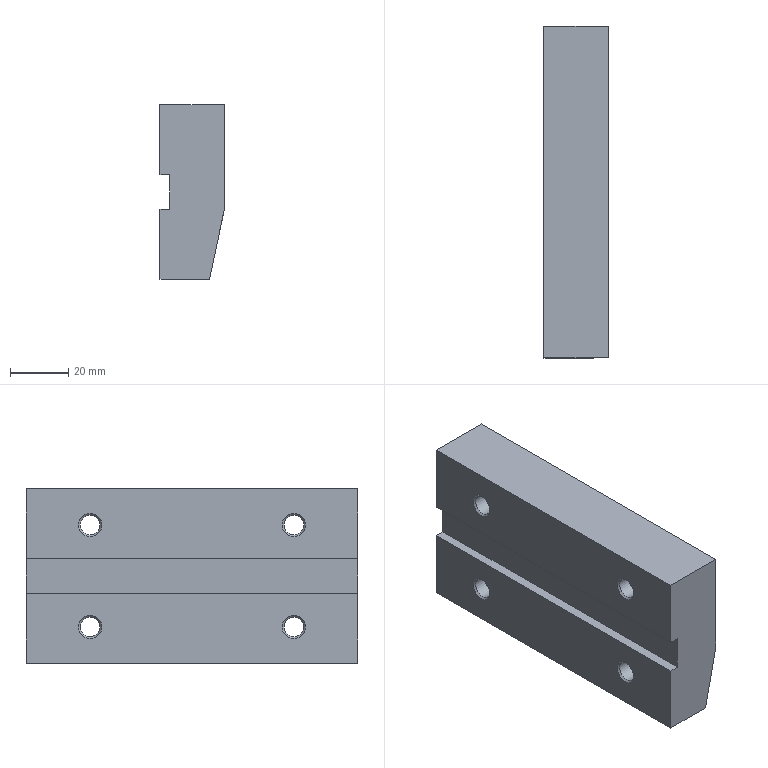Part | NX | features SIMPLE HOLE 4, SYMBOLIC_THREAD 4, DATUM_CSYS 3, SKETCH 2, EXTRUDE 1, HOLE PACKAGE 1 | 1 solid | 23 faces | box 22 x 114 x 60 mm | volume 136204 mm3 | plane 11 | cone 6 | cylinder 4 | spline 2 | commonest cylinder face diameters 6.8 x4
STEP:
#1=CARTESIAN_POINT('',(0.,92.,-51.5));
#2=VERTEX_POINT('',#1);
#3=CARTESIAN_POINT('',(0.,92.,-47.5));
#4=DIRECTION('',(1.,0.,0.));
#5=DIRECTION('',(0.,0.,-1.));
#6=AXIS2_PLACEMENT_3D('',#3,#4,#5);
#7=CIRCLE('',#6,4.);
#8=EDGE_CURVE('',#2,#2,#7,.T.);
#9=ORIENTED_EDGE('',*,*,#8,.T.);
#10=EDGE_LOOP('',(#9));
#11=FACE_BOUND('',#10,.T.);
#12=CARTESIAN_POINT('',(0.,22.,-51.5));
#13=VERTEX_POINT('',#12);
#14=CARTESIAN_POINT('',(0.,22.,-47.5));
#15=DIRECTION('',(1.,0.,0.));
#16=DIRECTION('',(0.,0.,-1.));
#17=AXIS2_PLACEMENT_3D('',#14,#15,#16);
#18=CIRCLE('',#17,4.);
#19=EDGE_CURVE('',#13,#13,#18,.T.);
#20=ORIENTED_EDGE('',*,*,#19,.T.);
#21=EDGE_LOOP('',(#20));
#22=FACE_BOUND('',#21,.T.);
#23=CARTESIAN_POINT('',(0.,0.,-60.));
#24=VERTEX_POINT('',#23);
#25=CARTESIAN_POINT('',(0.,0.,-36.));
#26=VERTEX_POINT('',#25);
#27=CARTESIAN_POINT('',(0.,0.,-60.));
#28=DIRECTION('',(0.,0.,1.));
#29=VECTOR('',#28,1000.);
#30=LINE('',#27,#29);
#31=EDGE_CURVE('',#24,#26,#30,.T.);
#32=ORIENTED_EDGE('',*,*,#31,.T.);
#33=CARTESIAN_POINT('',(0.,114.,-36.));
#34=VERTEX_POINT('',#33);
#35=CARTESIAN_POINT('',(0.,114.,-36.));
#36=DIRECTION('',(0.,-1.,0.));
#37=VECTOR('',#36,1000.);
#38=LINE('',#35,#37);
#39=EDGE_CURVE('',#34,#26,#38,.T.);
#40=ORIENTED_EDGE('',*,*,#39,.F.);
#41=CARTESIAN_POINT('',(0.,114.,-60.));
#42=VERTEX_POINT('',#41);
#43=CARTESIAN_POINT('',(0.,114.,-60.));
#44=DIRECTION('',(0.,0.,1.));
#45=VECTOR('',#44,1000.);
#46=LINE('',#43,#45);
#47=EDGE_CURVE('',#42,#34,#46,.T.);
#48=ORIENTED_EDGE('',*,*,#47,.F.);
#49=CARTESIAN_POINT('',(0.,114.,-60.));
#50=DIRECTION('',(0.,-1.,0.));
#51=VECTOR('',#50,1000.);
#52=LINE('',#49,#51);
#53=EDGE_CURVE('',#42,#24,#52,.T.);
#54=ORIENTED_EDGE('',*,*,#53,.T.);
#55=EDGE_LOOP('',(#32,#40,#48,#54));
#56=FACE_BOUND('',#55,.T.);
#57=CARTESIAN_POINT('',(0.,114.,-60.));
#58=DIRECTION('',(1.,0.,0.));
#59=DIRECTION('',(0.,0.,-1.));
#60=AXIS2_PLACEMENT_3D('',#57,#58,#59);
#61=PLANE('',#60);
#62=ADVANCED_FACE('',(#11,#22,#56),#61,.F.);
#63=CARTESIAN_POINT('',(3.3,0.,-36.));
#64=VERTEX_POINT('',#63);
#65=CARTESIAN_POINT('',(0.,0.,-36.));
#66=DIRECTION('',(1.,0.,0.));
#67=VECTOR('',#66,1000.);
#68=LINE('',#65,#67);
#69=EDGE_CURVE('',#26,#64,#68,.T.);
#70=ORIENTED_EDGE('',*,*,#69,.T.);
#71=CARTESIAN_POINT('',(3.3,114.,-36.));
#72=VERTEX_POINT('',#71);
#73=CARTESIAN_POINT('',(3.3,114.,-36.));
#74=DIRECTION('',(0.,-1.,0.));
#75=VECTOR('',#74,1000.);
#76=LINE('',#73,#75);
#77=EDGE_CURVE('',#72,#64,#76,.T.);
#78=ORIENTED_EDGE('',*,*,#77,.F.);
#79=CARTESIAN_POINT('',(0.,114.,-36.));
#80=DIRECTION('',(1.,0.,0.));
#81=VECTOR('',#80,1000.);
#82=LINE('',#79,#81);
#83=EDGE_CURVE('',#34,#72,#82,.T.);
#84=ORIENTED_EDGE('',*,*,#83,.F.);
#85=ORIENTED_EDGE('',*,*,#39,.T.);
#86=EDGE_LOOP('',(#70,#78,#84,#85));
#87=FACE_BOUND('',#86,.T.);
#88=CARTESIAN_POINT('',(0.,114.,-36.));
#89=DIRECTION('',(0.,0.,-1.));
#90=DIRECTION('',(-1.,0.,0.));
#91=AXIS2_PLACEMENT_3D('',#88,#89,#90);
#92=PLANE('',#91);
#93=ADVANCED_FACE('',(#87),#92,.F.);
#94=CARTESIAN_POINT('',(3.3,0.,-24.));
#95=VERTEX_POINT('',#94);
#96=CARTESIAN_POINT('',(3.3,0.,-36.));
#97=DIRECTION('',(0.,0.,1.));
#98=VECTOR('',#97,1000.);
#99=LINE('',#96,#98);
#100=EDGE_CURVE('',#64,#95,#99,.T.);
#101=ORIENTED_EDGE('',*,*,#100,.T.);
#102=CARTESIAN_POINT('',(3.3,114.,-24.));
#103=VERTEX_POINT('',#102);
#104=CARTESIAN_POINT('',(3.3,114.,-24.));
#105=DIRECTION('',(0.,-1.,0.));
#106=VECTOR('',#105,1000.);
#107=LINE('',#104,#106);
#108=EDGE_CURVE('',#103,#95,#107,.T.);
#109=ORIENTED_EDGE('',*,*,#108,.F.);
#110=CARTESIAN_POINT('',(3.3,114.,-36.));
#111=DIRECTION('',(0.,0.,1.));
#112=VECTOR('',#111,1000.);
#113=LINE('',#110,#112);
#114=EDGE_CURVE('',#72,#103,#113,.T.);
#115=ORIENTED_EDGE('',*,*,#114,.F.);
#116=ORIENTED_EDGE('',*,*,#77,.T.);
#117=EDGE_LOOP('',(#101,#109,#115,#116));
#118=FACE_BOUND('',#117,.T.);
#119=CARTESIAN_POINT('',(3.3,114.,-36.));
#120=DIRECTION('',(1.,0.,0.));
#121=DIRECTION('',(0.,0.,-1.));
#122=AXIS2_PLACEMENT_3D('',#119,#120,#121);
#123=PLANE('',#122);
#124=ADVANCED_FACE('',(#118),#123,.F.);
#125=CARTESIAN_POINT('',(0.,0.,-24.));
#126=VERTEX_POINT('',#125);
#127=CARTESIAN_POINT('',(3.3,0.,-24.));
#128=DIRECTION('',(-1.,0.,0.));
#129=VECTOR('',#128,1000.);
#130=LINE('',#127,#129);
#131=EDGE_CURVE('',#95,#126,#130,.T.);
#132=ORIENTED_EDGE('',*,*,#131,.T.);
#133=CARTESIAN_POINT('',(0.,114.,-24.));
#134=VERTEX_POINT('',#133);
#135=CARTESIAN_POINT('',(0.,114.,-24.));
#136=DIRECTION('',(0.,-1.,0.));
#137=VECTOR('',#136,1000.);
#138=LINE('',#135,#137);
#139=EDGE_CURVE('',#134,#126,#138,.T.);
#140=ORIENTED_EDGE('',*,*,#139,.F.);
#141=CARTESIAN_POINT('',(3.3,114.,-24.));
#142=DIRECTION('',(-1.,0.,0.));
#143=VECTOR('',#142,1000.);
#144=LINE('',#141,#143);
#145=EDGE_CURVE('',#103,#134,#144,.T.);
#146=ORIENTED_EDGE('',*,*,#145,.F.);
#147=ORIENTED_EDGE('',*,*,#108,.T.);
#148=EDGE_LOOP('',(#132,#140,#146,#147));
#149=FACE_BOUND('',#148,.T.);
#150=CARTESIAN_POINT('',(3.3,114.,-24.));
#151=DIRECTION('',(0.,0.,1.));
#152=DIRECTION('',(1.,0.,0.));
#153=AXIS2_PLACEMENT_3D('',#150,#151,#152);
#154=PLANE('',#153);
#155=ADVANCED_FACE('',(#149),#154,.F.);
#156=CARTESIAN_POINT('',(0.,92.,-16.5));
#157=VERTEX_POINT('',#156);
#158=CARTESIAN_POINT('',(0.,92.,-12.5));
#159=DIRECTION('',(1.,0.,0.));
#160=DIRECTION('',(0.,0.,-1.));
#161=AXIS2_PLACEMENT_3D('',#158,#159,#160);
#162=CIRCLE('',#161,4.);
#163=EDGE_CURVE('',#157,#157,#162,.T.);
#164=ORIENTED_EDGE('',*,*,#163,.T.);
#165=EDGE_LOOP('',(#164));
#166=FACE_BOUND('',#165,.T.);
#167=CARTESIAN_POINT('',(0.,22.,-16.5));
#168=VERTEX_POINT('',#167);
#169=CARTESIAN_POINT('',(0.,22.,-12.5));
#170=DIRECTION('',(1.,0.,0.));
#171=DIRECTION('',(0.,0.,-1.));
#172=AXIS2_PLACEMENT_3D('',#169,#170,#171);
#173=CIRCLE('',#172,4.);
#174=EDGE_CURVE('',#168,#168,#173,.T.);
#175=ORIENTED_EDGE('',*,*,#174,.T.);
#176=EDGE_LOOP('',(#175));
#177=FACE_BOUND('',#176,.T.);
#178=CARTESIAN_POINT('',(0.,0.,0.));
#179=VERTEX_POINT('',#178);
#180=CARTESIAN_POINT('',(0.,0.,-24.));
#181=DIRECTION('',(0.,0.,1.));
#182=VECTOR('',#181,1000.);
#183=LINE('',#180,#182);
#184=EDGE_CURVE('',#126,#179,#183,.T.);
#185=ORIENTED_EDGE('',*,*,#184,.T.);
#186=CARTESIAN_POINT('',(0.,114.,0.));
#187=VERTEX_POINT('',#186);
#188=CARTESIAN_POINT('',(0.,114.,0.));
#189=DIRECTION('',(0.,-1.,0.));
#190=VECTOR('',#189,1000.);
#191=LINE('',#188,#190);
#192=EDGE_CURVE('',#187,#179,#191,.T.);
#193=ORIENTED_EDGE('',*,*,#192,.F.);
#194=CARTESIAN_POINT('',(0.,114.,-24.));
#195=DIRECTION('',(0.,0.,1.));
#196=VECTOR('',#195,1000.);
#197=LINE('',#194,#196);
#198=EDGE_CURVE('',#134,#187,#197,.T.);
#199=ORIENTED_EDGE('',*,*,#198,.F.);
#200=ORIENTED_EDGE('',*,*,#139,.T.);
#201=EDGE_LOOP('',(#185,#193,#199,#200));
#202=FACE_BOUND('',#201,.T.);
#203=CARTESIAN_POINT('',(0.,114.,-24.));
#204=DIRECTION('',(1.,0.,0.));
#205=DIRECTION('',(0.,0.,-1.));
#206=AXIS2_PLACEMENT_3D('',#203,#204,#205);
#207=PLANE('',#206);
#208=ADVANCED_FACE('',(#166,#177,#202),#207,.F.);
#209=CARTESIAN_POINT('',(22.,0.,0.));
#210=VERTEX_POINT('',#209);
#211=CARTESIAN_POINT('',(0.,0.,0.));
#212=DIRECTION('',(1.,0.,0.));
#213=VECTOR('',#212,1000.);
#214=LINE('',#211,#213);
#215=EDGE_CURVE('',#179,#210,#214,.T.);
#216=ORIENTED_EDGE('',*,*,#215,.T.);
#217=CARTESIAN_POINT('',(22.,114.,0.));
#218=VERTEX_POINT('',#217);
#219=CARTESIAN_POINT('',(22.,114.,0.));
#220=DIRECTION('',(0.,-1.,0.));
#221=VECTOR('',#220,1000.);
#222=LINE('',#219,#221);
#223=EDGE_CURVE('',#218,#210,#222,.T.);
#224=ORIENTED_EDGE('',*,*,#223,.F.);
#225=CARTESIAN_POINT('',(0.,114.,0.));
#226=DIRECTION('',(1.,0.,0.));
#227=VECTOR('',#226,1000.);
#228=LINE('',#225,#227);
#229=EDGE_CURVE('',#187,#218,#228,.T.);
#230=ORIENTED_EDGE('',*,*,#229,.F.);
#231=ORIENTED_EDGE('',*,*,#192,.T.);
#232=EDGE_LOOP('',(#216,#224,#230,#231));
#233=FACE_BOUND('',#232,.T.);
#234=CARTESIAN_POINT('',(0.,114.,0.));
#235=DIRECTION('',(0.,0.,-1.));
#236=DIRECTION('',(-1.,0.,0.));
#237=AXIS2_PLACEMENT_3D('',#234,#235,#236);
#238=PLANE('',#237);
#239=ADVANCED_FACE('',(#233),#238,.F.);
#240=CARTESIAN_POINT('',(22.,92.,-8.5));
#241=VERTEX_POINT('',#240);
#242=CARTESIAN_POINT('',(22.,92.,-12.5));
#243=DIRECTION('',(-1.,0.,0.));
#244=DIRECTION('',(0.,0.,1.));
#245=AXIS2_PLACEMENT_3D('',#242,#243,#244);
#246=CIRCLE('',#245,4.);
#247=EDGE_CURVE('',#241,#241,#246,.T.);
#248=ORIENTED_EDGE('',*,*,#247,.T.);
#249=EDGE_LOOP('',(#248));
#250=FACE_BOUND('',#249,.T.);
#251=CARTESIAN_POINT('',(22.,22.,-8.5));
#252=VERTEX_POINT('',#251);
#253=CARTESIAN_POINT('',(22.,22.,-12.5));
#254=DIRECTION('',(-1.,0.,0.));
#255=DIRECTION('',(0.,0.,1.));
#256=AXIS2_PLACEMENT_3D('',#253,#254,#255);
#257=CIRCLE('',#256,4.);
#258=EDGE_CURVE('',#252,#252,#257,.T.);
#259=ORIENTED_EDGE('',*,*,#258,.T.);
#260=EDGE_LOOP('',(#259));
#261=FACE_BOUND('',#260,.T.);
#262=CARTESIAN_POINT('',(22.,0.,-36.477));
#263=VERTEX_POINT('',#262);
#264=CARTESIAN_POINT('',(22.,0.,0.));
#265=DIRECTION('',(0.,0.,-1.));
#266=VECTOR('',#265,1000.);
#267=LINE('',#264,#266);
#268=EDGE_CURVE('',#210,#263,#267,.T.);
#269=ORIENTED_EDGE('',*,*,#268,.T.);
#270=CARTESIAN_POINT('',(22.,114.,-36.477));
#271=VERTEX_POINT('',#270);
#272=CARTESIAN_POINT('',(22.,114.,-36.477));
#273=DIRECTION('',(0.,-1.,0.));
#274=VECTOR('',#273,1000.);
#275=LINE('',#272,#274);
#276=EDGE_CURVE('',#271,#263,#275,.T.);
#277=ORIENTED_EDGE('',*,*,#276,.F.);
#278=CARTESIAN_POINT('',(22.,114.,0.));
#279=DIRECTION('',(0.,0.,-1.));
#280=VECTOR('',#279,1000.);
#281=LINE('',#278,#280);
#282=EDGE_CURVE('',#218,#271,#281,.T.);
#283=ORIENTED_EDGE('',*,*,#282,.F.);
#284=ORIENTED_EDGE('',*,*,#223,.T.);
#285=EDGE_LOOP('',(#269,#277,#283,#284));
#286=FACE_BOUND('',#285,.T.);
#287=CARTESIAN_POINT('',(22.,114.,0.));
#288=DIRECTION('',(-1.,0.,0.));
#289=DIRECTION('',(0.,0.,1.));
#290=AXIS2_PLACEMENT_3D('',#287,#288,#289);
#291=PLANE('',#290);
#292=ADVANCED_FACE('',(#250,#261,#286),#291,.F.);
#293=CARTESIAN_POINT('',(20.479,92.,-43.632));
#294=VERTEX_POINT('',#293);
#295=CARTESIAN_POINT('',(20.43,90.379,-43.864));
#296=CARTESIAN_POINT('',(20.502,91.948,-43.525));
#297=CARTESIAN_POINT('',(20.437,93.507,-43.829));
#298=CARTESIAN_POINT('',(20.259,94.837,-44.667));
#299=CARTESIAN_POINT('',(19.981,95.74,-45.975));
#300=CARTESIAN_POINT('',(19.649,96.094,-47.536));
#301=CARTESIAN_POINT('',(19.317,95.807,-49.101));
#302=CARTESIAN_POINT('',(19.029,94.953,-50.456));
#303=CARTESIAN_POINT('',(18.837,93.644,-51.359));
#304=CARTESIAN_POINT('',(18.761,92.083,-51.713));
#305=CARTESIAN_POINT('',(18.822,90.518,-51.426));
#306=CARTESIAN_POINT('',(19.004,89.164,-50.573));
#307=CARTESIAN_POINT('',(19.282,88.261,-49.264));
#308=CARTESIAN_POINT('',(19.614,87.906,-47.703));
#309=CARTESIAN_POINT('',(19.946,88.193,-46.138));
#310=CARTESIAN_POINT('',(20.234,89.047,-44.784));
#311=CARTESIAN_POINT('',(20.43,90.379,-43.864));
#312=CARTESIAN_POINT('',(20.502,91.948,-43.525));
#313=CARTESIAN_POINT('',(20.437,93.507,-43.829));
#314=B_SPLINE_CURVE_WITH_KNOTS('',3,(#295,#296,#297,#298,#299,#300,#301,#302,#303,#304,#305,#306,#307,#308,#309,#310,#311,#312,#313),.UNSPECIFIED.,.T.,.F.,(1,1,1,1,1,1,1,1,1,1,1,1,1,1,1,1,1,1,1,1,1,1,1),(-0.1908,-0.1283,-0.06579,0.,0.05937,0.1217,0.1842,0.2467,0.3092,0.3717,0.4342,0.4967,0.5592,0.6217,0.6842,0.7467,0.8092,0.8717,0.9342,1.,1.059,1.122,1.184),.UNSPECIFIED.);
#315=EDGE_CURVE('',#294,#294,#314,.T.);
#316=ORIENTED_EDGE('',*,*,#315,.T.);
#317=EDGE_LOOP('',(#316));
#318=FACE_BOUND('',#317,.T.);
#319=CARTESIAN_POINT('',(20.479,22.,-43.632));
#320=VERTEX_POINT('',#319);
#321=CARTESIAN_POINT('',(20.43,20.379,-43.864));
#322=CARTESIAN_POINT('',(20.502,21.948,-43.525));
#323=CARTESIAN_POINT('',(20.437,23.507,-43.829));
#324=CARTESIAN_POINT('',(20.259,24.837,-44.667));
#325=CARTESIAN_POINT('',(19.981,25.74,-45.975));
#326=CARTESIAN_POINT('',(19.649,26.094,-47.536));
#327=CARTESIAN_POINT('',(19.317,25.807,-49.101));
#328=CARTESIAN_POINT('',(19.029,24.953,-50.456));
#329=CARTESIAN_POINT('',(18.837,23.644,-51.359));
#330=CARTESIAN_POINT('',(18.761,22.083,-51.713));
#331=CARTESIAN_POINT('',(18.822,20.518,-51.426));
#332=CARTESIAN_POINT('',(19.004,19.164,-50.573));
#333=CARTESIAN_POINT('',(19.282,18.261,-49.264));
#334=CARTESIAN_POINT('',(19.614,17.906,-47.703));
#335=CARTESIAN_POINT('',(19.946,18.193,-46.138));
#336=CARTESIAN_POINT('',(20.234,19.047,-44.784));
#337=CARTESIAN_POINT('',(20.43,20.379,-43.864));
#338=CARTESIAN_POINT('',(20.502,21.948,-43.525));
#339=CARTESIAN_POINT('',(20.437,23.507,-43.829));
#340=B_SPLINE_CURVE_WITH_KNOTS('',3,(#321,#322,#323,#324,#325,#326,#327,#328,#329,#330,#331,#332,#333,#334,#335,#336,#337,#338,#339),.UNSPECIFIED.,.T.,.F.,(1,1,1,1,1,1,1,1,1,1,1,1,1,1,1,1,1,1,1,1,1,1,1),(-0.1908,-0.1283,-0.06579,0.,0.05937,0.1217,0.1842,0.2467,0.3092,0.3717,0.4342,0.4967,0.5592,0.6217,0.6842,0.7467,0.8092,0.8717,0.9342,1.,1.059,1.122,1.184),.UNSPECIFIED.);
#341=EDGE_CURVE('',#320,#320,#340,.T.);
#342=ORIENTED_EDGE('',*,*,#341,.T.);
#343=EDGE_LOOP('',(#342));
#344=FACE_BOUND('',#343,.T.);
#345=CARTESIAN_POINT('',(17.,0.,-60.));
#346=VERTEX_POINT('',#345);
#347=CARTESIAN_POINT('',(22.,0.,-36.477));
#348=DIRECTION('',(-0.2079,0.,-0.9781));
#349=VECTOR('',#348,1000.);
#350=LINE('',#347,#349);
#351=EDGE_CURVE('',#263,#346,#350,.T.);
#352=ORIENTED_EDGE('',*,*,#351,.T.);
#353=CARTESIAN_POINT('',(17.,114.,-60.));
#354=VERTEX_POINT('',#353);
#355=CARTESIAN_POINT('',(17.,114.,-60.));
#356=DIRECTION('',(0.,-1.,0.));
#357=VECTOR('',#356,1000.);
#358=LINE('',#355,#357);
#359=EDGE_CURVE('',#354,#346,#358,.T.);
#360=ORIENTED_EDGE('',*,*,#359,.F.);
#361=CARTESIAN_POINT('',(22.,114.,-36.477));
#362=DIRECTION('',(-0.2079,0.,-0.9781));
#363=VECTOR('',#362,1000.);
#364=LINE('',#361,#363);
#365=EDGE_CURVE('',#271,#354,#364,.T.);
#366=ORIENTED_EDGE('',*,*,#365,.F.);
#367=ORIENTED_EDGE('',*,*,#276,.T.);
#368=EDGE_LOOP('',(#352,#360,#366,#367));
#369=FACE_BOUND('',#368,.T.);
#370=CARTESIAN_POINT('',(22.,114.,-36.477));
#371=DIRECTION('',(-0.9781,0.,0.2079));
#372=DIRECTION('',(0.2079,0.,0.9781));
#373=AXIS2_PLACEMENT_3D('',#370,#371,#372);
#374=PLANE('',#373);
#375=ADVANCED_FACE('',(#318,#344,#369),#374,.F.);
#376=CARTESIAN_POINT('',(17.,0.,-60.));
#377=DIRECTION('',(-1.,0.,0.));
#378=VECTOR('',#377,1000.);
#379=LINE('',#376,#378);
#380=EDGE_CURVE('',#346,#24,#379,.T.);
#381=ORIENTED_EDGE('',*,*,#380,.T.);
#382=ORIENTED_EDGE('',*,*,#53,.F.);
#383=CARTESIAN_POINT('',(17.,114.,-60.));
#384=DIRECTION('',(-1.,0.,0.));
#385=VECTOR('',#384,1000.);
#386=LINE('',#383,#385);
#387=EDGE_CURVE('',#354,#42,#386,.T.);
#388=ORIENTED_EDGE('',*,*,#387,.F.);
#389=ORIENTED_EDGE('',*,*,#359,.T.);
#390=EDGE_LOOP('',(#381,#382,#388,#389));
#391=FACE_BOUND('',#390,.T.);
#392=CARTESIAN_POINT('',(17.,114.,-60.));
#393=DIRECTION('',(0.,0.,1.));
#394=DIRECTION('',(1.,0.,0.));
#395=AXIS2_PLACEMENT_3D('',#392,#393,#394);
#396=PLANE('',#395);
#397=ADVANCED_FACE('',(#391),#396,.F.);
#398=ORIENTED_EDGE('',*,*,#47,.T.);
#399=ORIENTED_EDGE('',*,*,#83,.T.);
#400=ORIENTED_EDGE('',*,*,#114,.T.);
#401=ORIENTED_EDGE('',*,*,#145,.T.);
#402=ORIENTED_EDGE('',*,*,#198,.T.);
#403=ORIENTED_EDGE('',*,*,#229,.T.);
#404=ORIENTED_EDGE('',*,*,#282,.T.);
#405=ORIENTED_EDGE('',*,*,#365,.T.);
#406=ORIENTED_EDGE('',*,*,#387,.T.);
#407=EDGE_LOOP('',(#398,#399,#400,#401,#402,#403,#404,#405,#406));
#408=FACE_BOUND('',#407,.T.);
#409=CARTESIAN_POINT('',(0.,114.,0.));
#410=DIRECTION('',(0.,1.,0.));
#411=DIRECTION('',(0.,0.,1.));
#412=AXIS2_PLACEMENT_3D('',#409,#410,#411);
#413=PLANE('',#412);
#414=ADVANCED_FACE('',(#408),#413,.T.);
#415=ORIENTED_EDGE('',*,*,#31,.F.);
#416=ORIENTED_EDGE('',*,*,#380,.F.);
#417=ORIENTED_EDGE('',*,*,#351,.F.);
#418=ORIENTED_EDGE('',*,*,#268,.F.);
#419=ORIENTED_EDGE('',*,*,#215,.F.);
#420=ORIENTED_EDGE('',*,*,#184,.F.);
#421=ORIENTED_EDGE('',*,*,#131,.F.);
#422=ORIENTED_EDGE('',*,*,#100,.F.);
#423=ORIENTED_EDGE('',*,*,#69,.F.);
#424=EDGE_LOOP('',(#415,#416,#417,#418,#419,#420,#421,#422,#423));
#425=FACE_BOUND('',#424,.T.);
#426=CARTESIAN_POINT('',(0.,0.,0.));
#427=DIRECTION('',(0.,1.,0.));
#428=DIRECTION('',(0.,0.,1.));
#429=AXIS2_PLACEMENT_3D('',#426,#427,#428);
#430=PLANE('',#429);
#431=ADVANCED_FACE('',(#425),#430,.F.);
#432=CARTESIAN_POINT('',(19.917,22.,-44.1));
#433=VERTEX_POINT('',#432);
#434=CARTESIAN_POINT('',(19.882,23.125,-44.233));
#435=CARTESIAN_POINT('',(19.938,22.045,-44.019));
#436=CARTESIAN_POINT('',(19.887,20.98,-44.212));
#437=CARTESIAN_POINT('',(19.797,20.22,-44.574));
#438=CARTESIAN_POINT('',(19.687,19.644,-45.023));
#439=CARTESIAN_POINT('',(19.599,19.337,-45.369));
#440=CARTESIAN_POINT('',(19.433,18.886,-46.02));
#441=CARTESIAN_POINT('',(19.192,18.546,-47.006));
#442=CARTESIAN_POINT('',(18.898,18.637,-48.19));
#443=CARTESIAN_POINT('',(18.727,18.87,-48.887));
#444=CARTESIAN_POINT('',(18.584,19.202,-49.456));
#445=CARTESIAN_POINT('',(18.491,19.491,-49.817));
#446=CARTESIAN_POINT('',(18.376,20.,-50.281));
#447=CARTESIAN_POINT('',(18.264,20.798,-50.735));
#448=CARTESIAN_POINT('',(18.201,21.866,-50.979));
#449=CARTESIAN_POINT('',(18.243,22.939,-50.816));
#450=CARTESIAN_POINT('',(18.334,23.745,-50.45));
#451=CARTESIAN_POINT('',(18.448,24.345,-49.989));
#452=CARTESIAN_POINT('',(18.538,24.661,-49.634));
#453=CARTESIAN_POINT('',(18.704,25.112,-48.984));
#454=CARTESIAN_POINT('',(18.946,25.454,-47.996));
#455=CARTESIAN_POINT('',(19.24,25.363,-46.81));
#456=CARTESIAN_POINT('',(19.41,25.13,-46.113));
#457=CARTESIAN_POINT('',(19.554,24.798,-45.544));
#458=CARTESIAN_POINT('',(19.649,24.504,-45.177));
#459=CARTESIAN_POINT('',(19.768,23.971,-44.695));
#460=CARTESIAN_POINT('',(19.882,23.125,-44.233));
#461=CARTESIAN_POINT('',(19.938,22.045,-44.019));
#462=CARTESIAN_POINT('',(19.887,20.98,-44.212));
#463=B_SPLINE_CURVE_WITH_KNOTS('',3,(#434,#435,#436,#437,#438,#439,#440,#441,#442,#443,#444,#445,#446,#447,#448,#449,#450,#451,#452,#453,#454,#455,#456,#457,#458,#459,#460,#461,#462),.UNSPECIFIED.,.T.,.F.,(1,1,1,1,1,1,1,1,1,1,1,1,1,1,1,1,1,1,1,1,1,1,1,1,1,1,1,1,1,1,1,1,1),(-0.1316,-0.09868,-0.06579,0.,0.05937,0.08906,0.1187,0.1499,0.1811,0.2434,0.2747,0.3059,0.3372,0.3684,0.3997,0.4309,0.4934,0.5559,0.5872,0.6184,0.6497,0.6809,0.7434,0.7747,0.8059,0.8372,0.8684,0.9013,0.9342,1.,1.059,1.089,1.119),.UNSPECIFIED.);
#464=EDGE_CURVE('',#433,#433,#463,.T.);
#465=ORIENTED_EDGE('',*,*,#464,.T.);
#466=EDGE_LOOP('',(#465));
#467=FACE_BOUND('',#466,.T.);
#468=CARTESIAN_POINT('',(0.6,22.,-50.9));
#469=VERTEX_POINT('',#468);
#470=CARTESIAN_POINT('',(0.6,22.,-47.5));
#471=DIRECTION('',(1.,0.,0.));
#472=DIRECTION('',(0.,0.,-1.));
#473=AXIS2_PLACEMENT_3D('',#470,#471,#472);
#474=CIRCLE('',#473,3.4);
#475=EDGE_CURVE('',#469,#469,#474,.F.);
#476=ORIENTED_EDGE('',*,*,#475,.T.);
#477=EDGE_LOOP('',(#476));
#478=FACE_BOUND('',#477,.T.);
#479=CARTESIAN_POINT('',(0.,22.,-47.5));
#480=DIRECTION('',(1.,0.,0.));
#481=DIRECTION('',(0.,0.,-1.));
#482=AXIS2_PLACEMENT_3D('',#479,#480,#481);
#483=CYLINDRICAL_SURFACE('',#482,3.4);
#484=ADVANCED_FACE('',(#467,#478),#483,.F.);
#485=ORIENTED_EDGE('',*,*,#475,.F.);
#486=EDGE_LOOP('',(#485));
#487=FACE_BOUND('',#486,.T.);
#488=ORIENTED_EDGE('',*,*,#19,.F.);
#489=EDGE_LOOP('',(#488));
#490=FACE_BOUND('',#489,.T.);
#491=CARTESIAN_POINT('',(0.,22.,-47.5));
#492=DIRECTION('',(-1.,0.,0.));
#493=DIRECTION('',(0.,0.,1.));
#494=AXIS2_PLACEMENT_3D('',#491,#492,#493);
#495=CONICAL_SURFACE('',#494,4.,0.7854);
#496=ADVANCED_FACE('',(#487,#490),#495,.F.);
#497=ORIENTED_EDGE('',*,*,#464,.F.);
#498=EDGE_LOOP('',(#497));
#499=FACE_BOUND('',#498,.T.);
#500=ORIENTED_EDGE('',*,*,#341,.F.);
#501=EDGE_LOOP('',(#500));
#502=FACE_BOUND('',#501,.T.);
#503=CARTESIAN_POINT('',(20.479,20.955,-43.632));
#504=CARTESIAN_POINT('',(20.479,23.045,-43.632));
#505=CARTESIAN_POINT('',(20.388,24.081,-44.061));
#506=CARTESIAN_POINT('',(20.074,25.559,-45.539));
#507=CARTESIAN_POINT('',(19.854,25.988,-46.574));
#508=CARTESIAN_POINT('',(19.409,25.988,-48.665));
#509=CARTESIAN_POINT('',(19.189,25.559,-49.7));
#510=CARTESIAN_POINT('',(18.875,24.081,-51.179));
#511=CARTESIAN_POINT('',(18.784,23.045,-51.607));
#512=CARTESIAN_POINT('',(18.784,20.955,-51.607));
#513=CARTESIAN_POINT('',(18.875,19.919,-51.179));
#514=CARTESIAN_POINT('',(19.189,18.441,-49.7));
#515=CARTESIAN_POINT('',(19.409,18.012,-48.665));
#516=CARTESIAN_POINT('',(19.854,18.012,-46.574));
#517=CARTESIAN_POINT('',(20.074,18.441,-45.539));
#518=CARTESIAN_POINT('',(20.388,19.919,-44.061));
#519=CARTESIAN_POINT('',(20.479,20.955,-43.632));
#520=CARTESIAN_POINT('',(20.479,23.045,-43.632));
#521=CARTESIAN_POINT('',(19.917,21.109,-44.1));
#522=CARTESIAN_POINT('',(19.917,22.891,-44.1));
#523=CARTESIAN_POINT('',(19.825,23.774,-44.466));
#524=CARTESIAN_POINT('',(19.511,25.034,-45.726));
#525=CARTESIAN_POINT('',(19.291,25.4,-46.609));
#526=CARTESIAN_POINT('',(18.847,25.4,-48.391));
#527=CARTESIAN_POINT('',(18.627,25.034,-49.274));
#528=CARTESIAN_POINT('',(18.312,23.774,-50.534));
#529=CARTESIAN_POINT('',(18.221,22.891,-50.9));
#530=CARTESIAN_POINT('',(18.221,21.109,-50.9));
#531=CARTESIAN_POINT('',(18.312,20.226,-50.534));
#532=CARTESIAN_POINT('',(18.627,18.966,-49.274));
#533=CARTESIAN_POINT('',(18.847,18.6,-48.391));
#534=CARTESIAN_POINT('',(19.291,18.6,-46.609));
#535=CARTESIAN_POINT('',(19.511,18.966,-45.726));
#536=CARTESIAN_POINT('',(19.825,20.226,-44.466));
#537=CARTESIAN_POINT('',(19.917,21.109,-44.1));
#538=CARTESIAN_POINT('',(19.917,22.891,-44.1));
#539=B_SPLINE_SURFACE_WITH_KNOTS('',1,3,((#503,#504,#505,#506,#507,#508,#509,#510,#511,#512,#513,#514,#515,#516,#517,#518,#519,#520),(#521,#522,#523,#524,#525,#526,#527,#528,#529,#530,#531,#532,#533,#534,#535,#536,#537,#538)),.RULED_SURF.,.F.,.T.,.F.,(2,2),(2,2,2,2,2,2,2,2,2,2,2),(0.,1.),(-0.7854,0.,0.7854,1.571,2.356,3.142,3.927,4.712,5.498,6.283,7.069),.UNSPECIFIED.);
#540=ADVANCED_FACE('',(#499,#502),#539,.T.);
#541=CARTESIAN_POINT('',(21.4,22.,-9.1));
#542=VERTEX_POINT('',#541);
#543=CARTESIAN_POINT('',(21.4,22.,-12.5));
#544=DIRECTION('',(-1.,0.,0.));
#545=DIRECTION('',(0.,0.,1.));
#546=AXIS2_PLACEMENT_3D('',#543,#544,#545);
#547=CIRCLE('',#546,3.4);
#548=EDGE_CURVE('',#542,#542,#547,.F.);
#549=ORIENTED_EDGE('',*,*,#548,.T.);
#550=EDGE_LOOP('',(#549));
#551=FACE_BOUND('',#550,.T.);
#552=CARTESIAN_POINT('',(0.6,22.,-15.9));
#553=VERTEX_POINT('',#552);
#554=CARTESIAN_POINT('',(0.6,22.,-12.5));
#555=DIRECTION('',(1.,0.,0.));
#556=DIRECTION('',(0.,0.,-1.));
#557=AXIS2_PLACEMENT_3D('',#554,#555,#556);
#558=CIRCLE('',#557,3.4);
#559=EDGE_CURVE('',#553,#553,#558,.F.);
#560=ORIENTED_EDGE('',*,*,#559,.T.);
#561=EDGE_LOOP('',(#560));
#562=FACE_BOUND('',#561,.T.);
#563=CARTESIAN_POINT('',(0.,22.,-12.5));
#564=DIRECTION('',(1.,0.,0.));
#565=DIRECTION('',(0.,0.,-1.));
#566=AXIS2_PLACEMENT_3D('',#563,#564,#565);
#567=CYLINDRICAL_SURFACE('',#566,3.4);
#568=ADVANCED_FACE('',(#551,#562),#567,.F.);
#569=ORIENTED_EDGE('',*,*,#559,.F.);
#570=EDGE_LOOP('',(#569));
#571=FACE_BOUND('',#570,.T.);
#572=ORIENTED_EDGE('',*,*,#174,.F.);
#573=EDGE_LOOP('',(#572));
#574=FACE_BOUND('',#573,.T.);
#575=CARTESIAN_POINT('',(0.,22.,-12.5));
#576=DIRECTION('',(-1.,0.,0.));
#577=DIRECTION('',(0.,0.,1.));
#578=AXIS2_PLACEMENT_3D('',#575,#576,#577);
#579=CONICAL_SURFACE('',#578,4.,0.7854);
#580=ADVANCED_FACE('',(#571,#574),#579,.F.);
#581=ORIENTED_EDGE('',*,*,#548,.F.);
#582=EDGE_LOOP('',(#581));
#583=FACE_BOUND('',#582,.T.);
#584=ORIENTED_EDGE('',*,*,#258,.F.);
#585=EDGE_LOOP('',(#584));
#586=FACE_BOUND('',#585,.T.);
#587=CARTESIAN_POINT('',(22.,22.,-12.5));
#588=DIRECTION('',(1.,0.,0.));
#589=DIRECTION('',(0.,0.,-1.));
#590=AXIS2_PLACEMENT_3D('',#587,#588,#589);
#591=CONICAL_SURFACE('',#590,4.,0.7854);
#592=ADVANCED_FACE('',(#583,#586),#591,.F.);
#593=CARTESIAN_POINT('',(19.917,92.,-44.1));
#594=VERTEX_POINT('',#593);
#595=CARTESIAN_POINT('',(19.882,93.125,-44.233));
#596=CARTESIAN_POINT('',(19.938,92.045,-44.019));
#597=CARTESIAN_POINT('',(19.887,90.98,-44.212));
#598=CARTESIAN_POINT('',(19.797,90.22,-44.574));
#599=CARTESIAN_POINT('',(19.687,89.644,-45.023));
#600=CARTESIAN_POINT('',(19.599,89.337,-45.369));
#601=CARTESIAN_POINT('',(19.433,88.886,-46.02));
#602=CARTESIAN_POINT('',(19.192,88.546,-47.006));
#603=CARTESIAN_POINT('',(18.898,88.637,-48.19));
#604=CARTESIAN_POINT('',(18.727,88.87,-48.887));
#605=CARTESIAN_POINT('',(18.584,89.202,-49.456));
#606=CARTESIAN_POINT('',(18.491,89.491,-49.817));
#607=CARTESIAN_POINT('',(18.376,90.,-50.281));
#608=CARTESIAN_POINT('',(18.264,90.798,-50.735));
#609=CARTESIAN_POINT('',(18.201,91.866,-50.979));
#610=CARTESIAN_POINT('',(18.243,92.939,-50.816));
#611=CARTESIAN_POINT('',(18.334,93.745,-50.45));
#612=CARTESIAN_POINT('',(18.448,94.345,-49.989));
#613=CARTESIAN_POINT('',(18.538,94.661,-49.634));
#614=CARTESIAN_POINT('',(18.704,95.112,-48.984));
#615=CARTESIAN_POINT('',(18.946,95.454,-47.996));
#616=CARTESIAN_POINT('',(19.24,95.363,-46.81));
#617=CARTESIAN_POINT('',(19.41,95.13,-46.113));
#618=CARTESIAN_POINT('',(19.554,94.798,-45.544));
#619=CARTESIAN_POINT('',(19.649,94.504,-45.177));
#620=CARTESIAN_POINT('',(19.768,93.971,-44.695));
#621=CARTESIAN_POINT('',(19.882,93.125,-44.233));
#622=CARTESIAN_POINT('',(19.938,92.045,-44.019));
#623=CARTESIAN_POINT('',(19.887,90.98,-44.212));
#624=B_SPLINE_CURVE_WITH_KNOTS('',3,(#595,#596,#597,#598,#599,#600,#601,#602,#603,#604,#605,#606,#607,#608,#609,#610,#611,#612,#613,#614,#615,#616,#617,#618,#619,#620,#621,#622,#623),.UNSPECIFIED.,.T.,.F.,(1,1,1,1,1,1,1,1,1,1,1,1,1,1,1,1,1,1,1,1,1,1,1,1,1,1,1,1,1,1,1,1,1),(-0.1316,-0.09868,-0.06579,0.,0.05937,0.08906,0.1187,0.1499,0.1811,0.2434,0.2747,0.3059,0.3372,0.3684,0.3997,0.4309,0.4934,0.5559,0.5872,0.6184,0.6497,0.6809,0.7434,0.7747,0.8059,0.8372,0.8684,0.9013,0.9342,1.,1.059,1.089,1.119),.UNSPECIFIED.);
#625=EDGE_CURVE('',#594,#594,#624,.T.);
#626=ORIENTED_EDGE('',*,*,#625,.T.);
#627=EDGE_LOOP('',(#626));
#628=FACE_BOUND('',#627,.T.);
#629=CARTESIAN_POINT('',(0.6,92.,-50.9));
#630=VERTEX_POINT('',#629);
#631=CARTESIAN_POINT('',(0.6,92.,-47.5));
#632=DIRECTION('',(1.,0.,0.));
#633=DIRECTION('',(0.,0.,-1.));
#634=AXIS2_PLACEMENT_3D('',#631,#632,#633);
#635=CIRCLE('',#634,3.4);
#636=EDGE_CURVE('',#630,#630,#635,.F.);
#637=ORIENTED_EDGE('',*,*,#636,.T.);
#638=EDGE_LOOP('',(#637));
#639=FACE_BOUND('',#638,.T.);
#640=CARTESIAN_POINT('',(0.,92.,-47.5));
#641=DIRECTION('',(1.,0.,0.));
#642=DIRECTION('',(0.,0.,-1.));
#643=AXIS2_PLACEMENT_3D('',#640,#641,#642);
#644=CYLINDRICAL_SURFACE('',#643,3.4);
#645=ADVANCED_FACE('',(#628,#639),#644,.F.);
#646=ORIENTED_EDGE('',*,*,#636,.F.);
#647=EDGE_LOOP('',(#646));
#648=FACE_BOUND('',#647,.T.);
#649=ORIENTED_EDGE('',*,*,#8,.F.);
#650=EDGE_LOOP('',(#649));
#651=FACE_BOUND('',#650,.T.);
#652=CARTESIAN_POINT('',(0.,92.,-47.5));
#653=DIRECTION('',(-1.,0.,0.));
#654=DIRECTION('',(0.,0.,1.));
#655=AXIS2_PLACEMENT_3D('',#652,#653,#654);
#656=CONICAL_SURFACE('',#655,4.,0.7854);
#657=ADVANCED_FACE('',(#648,#651),#656,.F.);
#658=ORIENTED_EDGE('',*,*,#625,.F.);
#659=EDGE_LOOP('',(#658));
#660=FACE_BOUND('',#659,.T.);
#661=ORIENTED_EDGE('',*,*,#315,.F.);
#662=EDGE_LOOP('',(#661));
#663=FACE_BOUND('',#662,.T.);
#664=CARTESIAN_POINT('',(20.479,90.955,-43.632));
#665=CARTESIAN_POINT('',(20.479,93.045,-43.632));
#666=CARTESIAN_POINT('',(20.388,94.081,-44.061));
#667=CARTESIAN_POINT('',(20.074,95.559,-45.539));
#668=CARTESIAN_POINT('',(19.854,95.988,-46.574));
#669=CARTESIAN_POINT('',(19.409,95.988,-48.665));
#670=CARTESIAN_POINT('',(19.189,95.559,-49.7));
#671=CARTESIAN_POINT('',(18.875,94.081,-51.179));
#672=CARTESIAN_POINT('',(18.784,93.045,-51.607));
#673=CARTESIAN_POINT('',(18.784,90.955,-51.607));
#674=CARTESIAN_POINT('',(18.875,89.919,-51.179));
#675=CARTESIAN_POINT('',(19.189,88.441,-49.7));
#676=CARTESIAN_POINT('',(19.409,88.012,-48.665));
#677=CARTESIAN_POINT('',(19.854,88.012,-46.574));
#678=CARTESIAN_POINT('',(20.074,88.441,-45.539));
#679=CARTESIAN_POINT('',(20.388,89.919,-44.061));
#680=CARTESIAN_POINT('',(20.479,90.955,-43.632));
#681=CARTESIAN_POINT('',(20.479,93.045,-43.632));
#682=CARTESIAN_POINT('',(19.917,91.109,-44.1));
#683=CARTESIAN_POINT('',(19.917,92.891,-44.1));
#684=CARTESIAN_POINT('',(19.825,93.774,-44.466));
#685=CARTESIAN_POINT('',(19.511,95.034,-45.726));
#686=CARTESIAN_POINT('',(19.291,95.4,-46.609));
#687=CARTESIAN_POINT('',(18.847,95.4,-48.391));
#688=CARTESIAN_POINT('',(18.627,95.034,-49.274));
#689=CARTESIAN_POINT('',(18.312,93.774,-50.534));
#690=CARTESIAN_POINT('',(18.221,92.891,-50.9));
#691=CARTESIAN_POINT('',(18.221,91.109,-50.9));
#692=CARTESIAN_POINT('',(18.312,90.226,-50.534));
#693=CARTESIAN_POINT('',(18.627,88.966,-49.274));
#694=CARTESIAN_POINT('',(18.847,88.6,-48.391));
#695=CARTESIAN_POINT('',(19.291,88.6,-46.609));
#696=CARTESIAN_POINT('',(19.511,88.966,-45.726));
#697=CARTESIAN_POINT('',(19.825,90.226,-44.466));
#698=CARTESIAN_POINT('',(19.917,91.109,-44.1));
#699=CARTESIAN_POINT('',(19.917,92.891,-44.1));
#700=B_SPLINE_SURFACE_WITH_KNOTS('',1,3,((#664,#665,#666,#667,#668,#669,#670,#671,#672,#673,#674,#675,#676,#677,#678,#679,#680,#681),(#682,#683,#684,#685,#686,#687,#688,#689,#690,#691,#692,#693,#694,#695,#696,#697,#698,#699)),.RULED_SURF.,.F.,.T.,.F.,(2,2),(2,2,2,2,2,2,2,2,2,2,2),(0.,1.),(-0.7854,0.,0.7854,1.571,2.356,3.142,3.927,4.712,5.498,6.283,7.069),.UNSPECIFIED.);
#701=ADVANCED_FACE('',(#660,#663),#700,.T.);
#702=CARTESIAN_POINT('',(21.4,92.,-9.1));
#703=VERTEX_POINT('',#702);
#704=CARTESIAN_POINT('',(21.4,92.,-12.5));
#705=DIRECTION('',(-1.,0.,0.));
#706=DIRECTION('',(0.,0.,1.));
#707=AXIS2_PLACEMENT_3D('',#704,#705,#706);
#708=CIRCLE('',#707,3.4);
#709=EDGE_CURVE('',#703,#703,#708,.F.);
#710=ORIENTED_EDGE('',*,*,#709,.T.);
#711=EDGE_LOOP('',(#710));
#712=FACE_BOUND('',#711,.T.);
#713=CARTESIAN_POINT('',(0.6,92.,-15.9));
#714=VERTEX_POINT('',#713);
#715=CARTESIAN_POINT('',(0.6,92.,-12.5));
#716=DIRECTION('',(1.,0.,0.));
#717=DIRECTION('',(0.,0.,-1.));
#718=AXIS2_PLACEMENT_3D('',#715,#716,#717);
#719=CIRCLE('',#718,3.4);
#720=EDGE_CURVE('',#714,#714,#719,.F.);
#721=ORIENTED_EDGE('',*,*,#720,.T.);
#722=EDGE_LOOP('',(#721));
#723=FACE_BOUND('',#722,.T.);
#724=CARTESIAN_POINT('',(0.,92.,-12.5));
#725=DIRECTION('',(1.,0.,0.));
#726=DIRECTION('',(0.,0.,-1.));
#727=AXIS2_PLACEMENT_3D('',#724,#725,#726);
#728=CYLINDRICAL_SURFACE('',#727,3.4);
#729=ADVANCED_FACE('',(#712,#723),#728,.F.);
#730=ORIENTED_EDGE('',*,*,#720,.F.);
#731=EDGE_LOOP('',(#730));
#732=FACE_BOUND('',#731,.T.);
#733=ORIENTED_EDGE('',*,*,#163,.F.);
#734=EDGE_LOOP('',(#733));
#735=FACE_BOUND('',#734,.T.);
#736=CARTESIAN_POINT('',(0.,92.,-12.5));
#737=DIRECTION('',(-1.,0.,0.));
#738=DIRECTION('',(0.,0.,1.));
#739=AXIS2_PLACEMENT_3D('',#736,#737,#738);
#740=CONICAL_SURFACE('',#739,4.,0.7854);
#741=ADVANCED_FACE('',(#732,#735),#740,.F.);
#742=ORIENTED_EDGE('',*,*,#709,.F.);
#743=EDGE_LOOP('',(#742));
#744=FACE_BOUND('',#743,.T.);
#745=ORIENTED_EDGE('',*,*,#247,.F.);
#746=EDGE_LOOP('',(#745));
#747=FACE_BOUND('',#746,.T.);
#748=CARTESIAN_POINT('',(22.,92.,-12.5));
#749=DIRECTION('',(1.,0.,0.));
#750=DIRECTION('',(0.,0.,-1.));
#751=AXIS2_PLACEMENT_3D('',#748,#749,#750);
#752=CONICAL_SURFACE('',#751,4.,0.7854);
#753=ADVANCED_FACE('',(#744,#747),#752,.F.);
#754=CLOSED_SHELL('',(#62,#93,#124,#155,#208,#239,#292,#375,#397,#414,#431,#484,#496,#540,#568,#580,#592,#645,#657,#701,#729,#741,#753));
#755=MANIFOLD_SOLID_BREP('',#754);
#756=(LENGTH_UNIT()NAMED_UNIT(*)SI_UNIT(.MILLI.,.METRE.));
#757=UNCERTAINTY_MEASURE_WITH_UNIT(LENGTH_MEASURE(0.0508),#756,'','');
#758=(NAMED_UNIT(*)PLANE_ANGLE_UNIT()SI_UNIT($,.RADIAN.));
#759=(NAMED_UNIT(*)SI_UNIT($,.STERADIAN.)SOLID_ANGLE_UNIT());
#760=(GEOMETRIC_REPRESENTATION_CONTEXT(3)GLOBAL_UNCERTAINTY_ASSIGNED_CONTEXT((#757))GLOBAL_UNIT_ASSIGNED_CONTEXT((#756,#758,#759))REPRESENTATION_CONTEXT('',''));
#761=ADVANCED_BREP_SHAPE_REPRESENTATION('',(#755),#760);